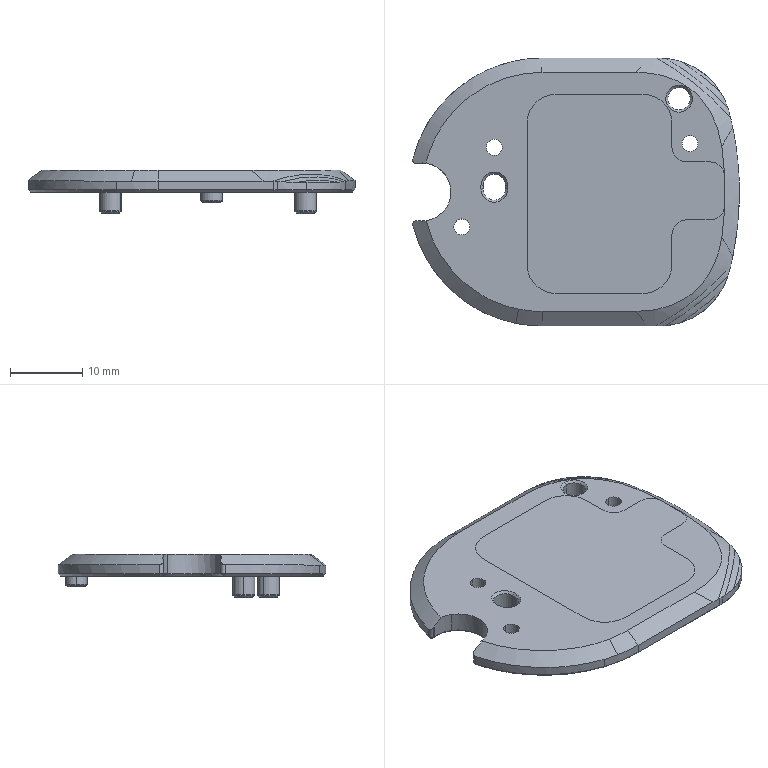NC program | NX | posted with a generic post | part box 45.101 x 36.973 x 6 mm
Lines 932 to 2608 of 3161, first 1365 of 1671 lines:
(ZLEVEL_PROFILE_COPY , TOOL : D2)
N1844 T17 M6
N1846 G54
N1848 G17 G0 G90 X-11.724 Y0.447 S9500 M3
N1850 G43 Z30. H17
N1852 Z1.5
N1854 G94 G1 Y0.253 Z1.49 F1000.
N1856 X-11.537 Y0.019 Z1.474
N1858 X-11.248 Y-0.059 Z1.458
N1860 X-10.941 Y0.074 Z1.441
N1862 X-10.824 Y0.253 Z1.429
N1864 Y1.087 Z1.386
N1866 X-10.941 Y1.266 Z1.375
N1868 X-11.247 Y1.399 Z1.357
N1870 X-11.537 Y1.322 Z1.341
N1872 X-11.724 Y1.087 Z1.326
N1874 Y0.253 Z1.282
N1876 X-11.537 Y0.019 Z1.266
N1878 X-11.248 Y-0.059 Z1.25
N1880 X-10.941 Y0.074 Z1.233
N1882 X-10.824 Y0.253 Z1.222
N1884 Y1.087 Z1.178
N1886 X-10.941 Y1.266 Z1.167
N1888 X-11.247 Y1.399 Z1.149
N1890 X-11.537 Y1.322 Z1.134
N1892 X-11.724 Y1.087 Z1.118
N1894 Y0.253 Z1.074
N1896 X-11.537 Y0.019 Z1.058
N1898 X-11.248 Y-0.059 Z1.043
N1900 X-10.941 Y0.074 Z1.025
N1902 X-10.824 Y0.253 Z1.014
N1904 Y1.087 Z0.97
N1906 X-10.941 Y1.266 Z0.959
N1908 X-11.247 Y1.399 Z0.942
N1910 X-11.537 Y1.322 Z0.926
N1912 X-11.724 Y1.087 Z0.91
N1914 Y0.253 Z0.866
N1916 X-11.537 Y0.019 Z0.851
N1918 X-11.248 Y-0.059 Z0.835
N1920 X-10.941 Y0.074 Z0.818
N1922 X-10.824 Y0.253 Z0.806
N1924 Y1.087 Z0.763
N1926 X-10.941 Y1.266 Z0.751
N1928 X-11.247 Y1.399 Z0.734
N1930 X-11.537 Y1.322 Z0.718
N1932 X-11.724 Y1.087 Z0.702
N1934 Y0.253 Z0.659
N1936 X-11.537 Y0.019 Z0.643
N1938 X-11.248 Y-0.059 Z0.627
N1940 X-10.941 Y0.074 Z0.61
N1942 X-10.824 Y0.253 Z0.599
N1944 Y1.087 Z0.555
N1946 X-10.941 Y1.266 Z0.544
N1948 X-11.247 Y1.399 Z0.526
N1950 X-11.537 Y1.322 Z0.511
N1952 X-11.724 Y1.087 Z0.495
N1954 Y0.253 Z0.451
N1956 X-11.537 Y0.019 Z0.435
N1958 X-11.248 Y-0.059 Z0.42
N1960 X-10.941 Y0.074 Z0.402
N1962 X-10.824 Y0.253 Z0.391
N1964 Y1.087 Z0.347
N1966 X-10.941 Y1.266 Z0.336
N1968 X-11.247 Y1.399 Z0.319
N1970 X-11.537 Y1.322 Z0.303
N1972 X-11.724 Y1.087 Z0.287
N1974 Y0.253 Z0.243
N1976 X-11.537 Y0.019 Z0.228
N1978 X-11.248 Y-0.059 Z0.212
N1980 X-10.941 Y0.074 Z0.194
N1982 X-10.824 Y0.253 Z0.183
N1984 Y1.087 Z0.14
N1986 X-10.941 Y1.266 Z0.128
N1988 X-11.247 Y1.399 Z0.111
N1990 X-11.537 Y1.322 Z0.095
N1992 X-11.724 Y1.087 Z0.079
N1994 Y0.253 Z0.036
N1996 X-11.537 Y0.019 Z0.02
N1998 X-11.248 Y-0.059 Z0.004
N2000 X-10.941 Y0.074 Z-0.013
N2002 X-10.824 Y0.253 Z-0.024
N2004 Y1.087 Z-0.068
N2006 X-10.941 Y1.266 Z-0.079
N2008 X-11.247 Y1.399 Z-0.097
N2010 X-11.537 Y1.322 Z-0.113
N2012 X-11.724 Y1.087 Z-0.128
N2014 Y0.67 Z-0.15
N2016 Y0.42 F1200.
N2018 G3 X-11.274 Y-0.03 R0.45
N2020 X-10.824 Y0.42 R0.45
N2022 G1 Y0.92
N2024 G3 X-11.274 Y1.37 R0.45
N2026 X-11.724 Y0.92 R0.45
N2028 G1 Y0.67
N2030 X-11.703 Y0.42 Z-0.163
N2032 X-11.692 Y0.356 Z-0.167
N2034 X-11.614 Y0.17 Z-0.178
N2036 X-11.551 Y0.097 Z-0.184
N2038 X-11.392 Y0.013 Z-0.193
N2040 X-11.274 Y-0.011 Z-0.2
N2042 X-11.111 Y0.022 Z-0.209
N2044 X-10.997 Y0.097 Z-0.217
N2046 X-10.912 Y0.202 Z-0.224
N2048 X-10.857 Y0.356 Z-0.234
N2050 X-10.83 Y0.498 Z-0.241
N2052 X-10.824 Y0.67 Z-0.25
N2054 Y0.909 Z-0.263
N2056 X-10.857 Y0.985 Z-0.267
N2058 X-10.967 Y1.219 Z-0.281
N2060 X-10.997 Y1.243 Z-0.284
N2062 X-11.13 Y1.322 Z-0.292
N2064 X-11.274 Y1.37 Z-0.3
N2066 G3 X-11.724 Y0.92 R0.45
N2068 G1 Y0.67
N2070 X-11.703 Y0.42 Z-0.313
N2072 X-11.692 Y0.356 Z-0.317
N2074 X-11.614 Y0.17 Z-0.328
N2076 X-11.551 Y0.097 Z-0.334
N2078 X-11.392 Y0.013 Z-0.343
N2080 X-11.274 Y-0.011 Z-0.35
N2082 X-11.111 Y0.022 Z-0.359
N2084 X-10.997 Y0.097 Z-0.367
N2086 X-10.912 Y0.202 Z-0.374
N2088 X-10.857 Y0.356 Z-0.384
N2090 X-10.83 Y0.498 Z-0.391
N2092 X-10.824 Y0.67 Z-0.4
N2094 Y0.909 Z-0.413
N2096 X-10.857 Y0.985 Z-0.417
N2098 X-10.967 Y1.219 Z-0.431
N2100 X-10.997 Y1.243 Z-0.434
N2102 X-11.13 Y1.322 Z-0.442
N2104 X-11.274 Y1.37 Z-0.45
N2106 G3 X-11.724 Y0.92 R0.45
N2108 G1 Y0.67
N2110 X-11.703 Y0.42 Z-0.463
N2112 X-11.692 Y0.356 Z-0.467
N2114 X-11.614 Y0.17 Z-0.478
N2116 X-11.551 Y0.097 Z-0.484
N2118 X-11.392 Y0.013 Z-0.493
N2120 X-11.274 Y-0.011 Z-0.5
N2122 X-11.111 Y0.022 Z-0.509
N2124 X-10.997 Y0.097 Z-0.517
N2126 X-10.912 Y0.202 Z-0.524
N2128 X-10.857 Y0.356 Z-0.534
N2130 X-10.83 Y0.498 Z-0.541
N2132 X-10.824 Y0.67 Z-0.55
N2134 Y0.909 Z-0.563
N2136 X-10.857 Y0.985 Z-0.567
N2138 X-10.967 Y1.219 Z-0.581
N2140 X-10.997 Y1.243 Z-0.584
N2142 X-11.13 Y1.322 Z-0.592
N2144 X-11.274 Y1.37 Z-0.6
N2146 G3 X-11.724 Y0.92 R0.45
N2148 G1 Y0.67
N2150 X-11.703 Y0.42 Z-0.613
N2152 X-11.692 Y0.356 Z-0.617
N2154 X-11.614 Y0.17 Z-0.628
N2156 X-11.551 Y0.097 Z-0.634
N2158 X-11.392 Y0.013 Z-0.643
N2160 X-11.274 Y-0.011 Z-0.65
N2162 X-11.111 Y0.022 Z-0.659
N2164 X-10.997 Y0.097 Z-0.667
N2166 X-10.912 Y0.202 Z-0.674
N2168 X-10.857 Y0.356 Z-0.684
N2170 X-10.83 Y0.498 Z-0.691
N2172 X-10.824 Y0.67 Z-0.7
N2174 Y0.909 Z-0.713
N2176 X-10.857 Y0.985 Z-0.717
N2178 X-10.967 Y1.219 Z-0.731
N2180 X-10.997 Y1.243 Z-0.734
N2182 X-11.13 Y1.322 Z-0.742
N2184 X-11.274 Y1.37 Z-0.75
N2186 G3 X-11.724 Y0.92 R0.45
N2188 G1 Y0.67
N2190 X-11.703 Y0.42 Z-0.763
N2192 X-11.692 Y0.356 Z-0.767
N2194 X-11.614 Y0.17 Z-0.778
N2196 X-11.551 Y0.097 Z-0.784
N2198 X-11.392 Y0.013 Z-0.793
N2200 X-11.274 Y-0.011 Z-0.8
N2202 X-11.111 Y0.022 Z-0.809
N2204 X-10.997 Y0.097 Z-0.817
N2206 X-10.912 Y0.202 Z-0.824
N2208 X-10.857 Y0.356 Z-0.834
N2210 X-10.83 Y0.498 Z-0.841
N2212 X-10.824 Y0.67 Z-0.85
N2214 Y0.909 Z-0.863
N2216 X-10.857 Y0.985 Z-0.867
N2218 X-10.967 Y1.219 Z-0.881
N2220 X-10.997 Y1.243 Z-0.884
N2222 X-11.13 Y1.322 Z-0.892
N2224 X-11.274 Y1.37 Z-0.9
N2226 G3 X-11.724 Y0.92 R0.45
N2228 G1 Y0.67
N2230 X-11.703 Y0.42 Z-0.913
N2232 X-11.692 Y0.356 Z-0.917
N2234 X-11.614 Y0.17 Z-0.928
N2236 X-11.551 Y0.097 Z-0.934
N2238 X-11.392 Y0.013 Z-0.943
N2240 X-11.274 Y-0.011 Z-0.95
N2242 X-11.111 Y0.022 Z-0.959
N2244 X-10.997 Y0.097 Z-0.967
N2246 X-10.912 Y0.202 Z-0.974
N2248 X-10.857 Y0.356 Z-0.984
N2250 X-10.83 Y0.498 Z-0.991
N2252 X-10.824 Y0.67 Z-1.
N2254 Y0.909 Z-1.013
N2256 X-10.857 Y0.985 Z-1.017
N2258 X-10.967 Y1.219 Z-1.031
N2260 X-10.997 Y1.243 Z-1.034
N2262 X-11.13 Y1.322 Z-1.042
N2264 X-11.274 Y1.37 Z-1.05
N2266 G3 X-11.724 Y0.92 R0.45
N2268 G1 Y0.67
N2270 X-11.703 Y0.42 Z-1.063
N2272 X-11.692 Y0.356 Z-1.067
N2274 X-11.614 Y0.17 Z-1.078
N2276 X-11.551 Y0.097 Z-1.084
N2278 X-11.392 Y0.013 Z-1.093
N2280 X-11.274 Y-0.011 Z-1.1
N2282 X-11.111 Y0.022 Z-1.109
N2284 X-10.997 Y0.097 Z-1.117
N2286 X-10.912 Y0.202 Z-1.124
N2288 X-10.857 Y0.356 Z-1.134
N2290 X-10.83 Y0.498 Z-1.141
N2292 X-10.824 Y0.67 Z-1.15
N2294 Y0.909 Z-1.163
N2296 X-10.857 Y0.985 Z-1.167
N2298 X-10.967 Y1.219 Z-1.181
N2300 X-10.997 Y1.243 Z-1.184
N2302 X-11.13 Y1.322 Z-1.192
N2304 X-11.274 Y1.37 Z-1.2
N2306 G3 X-11.724 Y0.92 R0.45
N2308 G1 Y0.67
N2310 X-11.703 Y0.42 Z-1.213
N2312 X-11.692 Y0.356 Z-1.217
N2314 X-11.614 Y0.17 Z-1.228
N2316 X-11.551 Y0.097 Z-1.234
N2318 X-11.392 Y0.013 Z-1.243
N2320 X-11.274 Y-0.011 Z-1.25
N2322 X-11.111 Y0.022 Z-1.259
N2324 X-10.997 Y0.097 Z-1.267
N2326 X-10.912 Y0.202 Z-1.274
N2328 X-10.857 Y0.356 Z-1.284
N2330 X-10.83 Y0.498 Z-1.291
N2332 X-10.824 Y0.67 Z-1.3
N2334 Y0.909 Z-1.313
N2336 X-10.857 Y0.985 Z-1.317
N2338 X-10.967 Y1.219 Z-1.331
N2340 X-10.997 Y1.243 Z-1.334
N2342 X-11.13 Y1.322 Z-1.342
N2344 X-11.274 Y1.37 Z-1.35
N2346 G3 X-11.724 Y0.92 R0.45
N2348 G1 Y0.67
N2350 X-11.703 Y0.42 Z-1.363
N2352 X-11.692 Y0.356 Z-1.367
N2354 X-11.614 Y0.17 Z-1.378
N2356 X-11.551 Y0.097 Z-1.384
N2358 X-11.392 Y0.013 Z-1.393
N2360 X-11.274 Y-0.011 Z-1.4
N2362 X-11.111 Y0.022 Z-1.409
N2364 X-10.997 Y0.097 Z-1.417
N2366 X-10.912 Y0.202 Z-1.424
N2368 X-10.857 Y0.356 Z-1.434
N2370 X-10.83 Y0.498 Z-1.441
N2372 X-10.824 Y0.67 Z-1.45
N2374 Y0.909 Z-1.463
N2376 X-10.857 Y0.985 Z-1.467
N2378 X-10.967 Y1.219 Z-1.481
N2380 X-10.997 Y1.243 Z-1.484
N2382 X-11.13 Y1.322 Z-1.492
N2384 X-11.274 Y1.37 Z-1.5
N2386 G3 X-11.724 Y0.92 R0.45
N2388 G1 Y0.67
N2390 X-11.703 Y0.42 Z-1.513
N2392 X-11.692 Y0.356 Z-1.517
N2394 X-11.614 Y0.17 Z-1.528
N2396 X-11.551 Y0.097 Z-1.534
N2398 X-11.392 Y0.013 Z-1.543
N2400 X-11.274 Y-0.011 Z-1.55
N2402 X-11.111 Y0.022 Z-1.559
N2404 X-10.997 Y0.097 Z-1.567
N2406 X-10.912 Y0.202 Z-1.574
N2408 X-10.857 Y0.356 Z-1.584
N2410 X-10.83 Y0.498 Z-1.591
N2412 X-10.824 Y0.67 Z-1.6
N2414 Y0.909 Z-1.613
N2416 X-10.857 Y0.985 Z-1.617
N2418 X-10.967 Y1.219 Z-1.631
N2420 X-10.997 Y1.243 Z-1.634
N2422 X-11.13 Y1.322 Z-1.642
N2424 X-11.274 Y1.37 Z-1.65
N2426 G3 X-11.724 Y0.92 R0.45
N2428 G1 Y0.67
N2430 X-11.703 Y0.42 Z-1.663
N2432 X-11.692 Y0.356 Z-1.667
N2434 X-11.614 Y0.17 Z-1.678
N2436 X-11.551 Y0.097 Z-1.684
N2438 X-11.392 Y0.013 Z-1.693
N2440 X-11.274 Y-0.011 Z-1.7
N2442 X-11.111 Y0.022 Z-1.709
N2444 X-10.997 Y0.097 Z-1.717
N2446 X-10.912 Y0.202 Z-1.724
N2448 X-10.857 Y0.356 Z-1.734
N2450 X-10.83 Y0.498 Z-1.741
N2452 X-10.824 Y0.67 Z-1.75
N2454 Y0.909 Z-1.763
N2456 X-10.857 Y0.985 Z-1.767
N2458 X-10.967 Y1.219 Z-1.781
N2460 X-10.997 Y1.243 Z-1.784
N2462 X-11.13 Y1.322 Z-1.792
N2464 X-11.274 Y1.37 Z-1.8
N2466 G3 X-11.724 Y0.92 R0.45
N2468 G1 Y0.67
N2470 X-11.703 Y0.42 Z-1.813
N2472 X-11.692 Y0.356 Z-1.817
N2474 X-11.614 Y0.17 Z-1.828
N2476 X-11.551 Y0.097 Z-1.834
N2478 X-11.392 Y0.013 Z-1.843
N2480 X-11.274 Y-0.011 Z-1.85
N2482 X-11.111 Y0.022 Z-1.859
N2484 X-10.997 Y0.097 Z-1.867
N2486 X-10.912 Y0.202 Z-1.874
N2488 X-10.857 Y0.356 Z-1.884
N2490 X-10.83 Y0.498 Z-1.891
N2492 X-10.824 Y0.67 Z-1.9
N2494 Y0.909 Z-1.913
N2496 X-10.857 Y0.985 Z-1.917
N2498 X-10.967 Y1.219 Z-1.931
N2500 X-10.997 Y1.243 Z-1.934
N2502 X-11.13 Y1.322 Z-1.942
N2504 X-11.274 Y1.37 Z-1.95
N2506 G3 X-11.724 Y0.92 R0.45
N2508 G1 Y0.67
N2510 X-11.703 Y0.42 Z-1.963
N2512 X-11.692 Y0.356 Z-1.967
N2514 X-11.614 Y0.17 Z-1.978
N2516 X-11.551 Y0.097 Z-1.984
N2518 X-11.392 Y0.013 Z-1.993
N2520 X-11.274 Y-0.011 Z-2.
N2522 X-11.111 Y0.022 Z-2.009
N2524 X-10.997 Y0.097 Z-2.017
N2526 X-10.912 Y0.202 Z-2.024
N2528 X-10.857 Y0.356 Z-2.034
N2530 X-10.83 Y0.498 Z-2.041
N2532 X-10.824 Y0.67 Z-2.05
N2534 Y0.909 Z-2.063
N2536 X-10.857 Y0.985 Z-2.067
N2538 X-10.967 Y1.219 Z-2.081
N2540 X-10.997 Y1.243 Z-2.084
N2542 X-11.13 Y1.322 Z-2.092
N2544 X-11.274 Y1.37 Z-2.1
N2546 G3 X-11.724 Y0.92 R0.45
N2548 G1 Y0.67
N2550 X-11.703 Y0.42 Z-2.113
N2552 X-11.692 Y0.356 Z-2.117
N2554 X-11.614 Y0.17 Z-2.128
N2556 X-11.551 Y0.097 Z-2.134
N2558 X-11.392 Y0.013 Z-2.143
N2560 X-11.274 Y-0.011 Z-2.15
N2562 X-11.111 Y0.022 Z-2.159
N2564 X-10.997 Y0.097 Z-2.167
N2566 X-10.912 Y0.202 Z-2.174
N2568 X-10.857 Y0.356 Z-2.184
N2570 X-10.83 Y0.498 Z-2.191
N2572 X-10.824 Y0.67 Z-2.2
N2574 Y0.909 Z-2.213
N2576 X-10.857 Y0.985 Z-2.217
N2578 X-10.967 Y1.219 Z-2.231
N2580 X-10.997 Y1.243 Z-2.234
N2582 X-11.13 Y1.322 Z-2.242
N2584 X-11.274 Y1.37 Z-2.25
N2586 G3 X-11.724 Y0.92 R0.45
N2588 G1 Y0.67
N2590 X-11.703 Y0.42 Z-2.263
N2592 X-11.692 Y0.356 Z-2.267
N2594 X-11.614 Y0.17 Z-2.278
N2596 X-11.551 Y0.097 Z-2.284
N2598 X-11.392 Y0.013 Z-2.293
N2600 X-11.274 Y-0.011 Z-2.3
N2602 X-11.111 Y0.022 Z-2.309
N2604 X-10.997 Y0.097 Z-2.317
N2606 X-10.912 Y0.202 Z-2.324
N2608 X-10.857 Y0.356 Z-2.334
N2610 X-10.83 Y0.498 Z-2.341
N2612 X-10.824 Y0.67 Z-2.35
N2614 Y0.909 Z-2.363
N2616 X-10.857 Y0.985 Z-2.367
N2618 X-10.967 Y1.219 Z-2.381
N2620 X-10.997 Y1.243 Z-2.384
N2622 X-11.13 Y1.322 Z-2.392
N2624 X-11.274 Y1.37 Z-2.4
N2626 G3 X-11.724 Y0.92 R0.45
N2628 G1 Y0.67
N2630 X-11.703 Y0.42 Z-2.413
N2632 X-11.692 Y0.356 Z-2.417
N2634 X-11.614 Y0.17 Z-2.428
N2636 X-11.551 Y0.097 Z-2.434
N2638 X-11.392 Y0.013 Z-2.443
N2640 X-11.274 Y-0.011 Z-2.45
N2642 X-11.111 Y0.022 Z-2.459
N2644 X-10.997 Y0.097 Z-2.467
N2646 X-10.912 Y0.202 Z-2.474
N2648 X-10.857 Y0.356 Z-2.484
N2650 X-10.83 Y0.498 Z-2.491
N2652 X-10.824 Y0.67 Z-2.5
N2654 Y0.909 Z-2.513
N2656 X-10.857 Y0.985 Z-2.517
N2658 X-10.967 Y1.219 Z-2.531
N2660 X-10.997 Y1.243 Z-2.534
N2662 X-11.13 Y1.322 Z-2.542
N2664 X-11.274 Y1.37 Z-2.55
N2666 G3 X-11.724 Y0.92 R0.45
N2668 G1 Y0.67
N2670 X-11.703 Y0.42 Z-2.563
N2672 X-11.692 Y0.356 Z-2.567
N2674 X-11.614 Y0.17 Z-2.578
N2676 X-11.551 Y0.097 Z-2.584
N2678 X-11.392 Y0.013 Z-2.593
N2680 X-11.274 Y-0.011 Z-2.6
N2682 X-11.111 Y0.022 Z-2.609
N2684 X-10.997 Y0.097 Z-2.617
N2686 X-10.912 Y0.202 Z-2.624
N2688 X-10.857 Y0.356 Z-2.634
N2690 X-10.83 Y0.498 Z-2.641
N2692 X-10.824 Y0.67 Z-2.65
N2694 Y0.909 Z-2.663
N2696 X-10.857 Y0.985 Z-2.667
N2698 X-10.967 Y1.219 Z-2.681
N2700 X-10.997 Y1.243 Z-2.684
N2702 X-11.13 Y1.322 Z-2.692
N2704 X-11.274 Y1.37 Z-2.7
N2706 G3 X-11.724 Y0.92 R0.45
N2708 G1 Y0.67
N2710 X-11.703 Y0.42 Z-2.713
N2712 X-11.692 Y0.356 Z-2.717
N2714 X-11.614 Y0.17 Z-2.728
N2716 X-11.551 Y0.097 Z-2.734
N2718 X-11.392 Y0.013 Z-2.743
N2720 X-11.274 Y-0.011 Z-2.75
N2722 X-11.111 Y0.022 Z-2.759
N2724 X-10.997 Y0.097 Z-2.767
N2726 X-10.912 Y0.202 Z-2.774
N2728 X-10.857 Y0.356 Z-2.784
N2730 X-10.83 Y0.498 Z-2.791
N2732 X-10.824 Y0.67 Z-2.8
N2734 Y0.909 Z-2.813
N2736 X-10.857 Y0.985 Z-2.817
N2738 X-10.967 Y1.219 Z-2.831
N2740 X-10.997 Y1.243 Z-2.834
N2742 X-11.13 Y1.322 Z-2.842
N2744 X-11.274 Y1.37 Z-2.85
N2746 G3 X-11.724 Y0.92 R0.45
N2748 G1 Y0.67
N2750 X-11.703 Y0.42 Z-2.863
N2752 X-11.692 Y0.356 Z-2.867
N2754 X-11.614 Y0.17 Z-2.878
N2756 X-11.551 Y0.097 Z-2.884
N2758 X-11.392 Y0.013 Z-2.893
N2760 X-11.274 Y-0.011 Z-2.9
N2762 X-11.111 Y0.022 Z-2.909
N2764 X-10.997 Y0.097 Z-2.917
N2766 X-10.912 Y0.202 Z-2.924
N2768 X-10.857 Y0.356 Z-2.934
N2770 X-10.83 Y0.498 Z-2.941
N2772 X-10.824 Y0.67 Z-2.95
N2774 Y0.909 Z-2.963
N2776 X-10.857 Y0.985 Z-2.967
N2778 X-10.967 Y1.219 Z-2.981
N2780 X-10.997 Y1.243 Z-2.984
N2782 X-11.13 Y1.322 Z-2.992
N2784 X-11.274 Y1.37 Z-3.
N2786 G3 X-11.724 Y0.92 R0.45
N2788 G1 Y0.42
N2790 G3 X-11.274 Y-0.03 R0.45
N2792 X-10.824 Y0.42 R0.45
N2794 G1 Y0.92
N2796 G3 X-11.274 Y1.37 R0.45
N2798 G1 Z-1.5
N2800 G0 Z30.
N2802 X13.893 Y12.55
N2804 Z1.5
N2806 G1 X14.081 Y12.412 Z1.488 F1000.
N2808 X14.415 Y12.429 Z1.47
N2810 X14.633 Y12.615 Z1.455
N2812 X14.705 Y12.892 Z1.44
N2814 X14.575 Y13.2 Z1.423
N2816 X14.415 Y13.311 Z1.412
N2818 X14.226 Y13.32 Z1.402
N2820 X14.059 Z1.394
N2822 X13.877 Y13.2 Z1.382
N2824 X13.746 Y12.892 Z1.365
N2826 X13.832 Y12.595 Z1.349
N2828 X14.081 Y12.412 Z1.332
N2830 X14.415 Y12.429 Z1.315
N2832 X14.633 Y12.615 Z1.3
N2834 X14.705 Y12.892 Z1.285
N2836 X14.575 Y13.2 Z1.267
N2838 X14.415 Y13.311 Z1.257
N2840 X14.226 Y13.32 Z1.247
N2842 X14.059 Z1.238
N2844 X13.877 Y13.2 Z1.227
N2846 X13.746 Y12.892 Z1.209
N2848 X13.832 Y12.595 Z1.193
N2850 X14.081 Y12.412 Z1.177
N2852 X14.415 Y12.429 Z1.16
N2854 X14.633 Y12.615 Z1.145
N2856 X14.705 Y12.892 Z1.13
N2858 X14.575 Y13.2 Z1.112
N2860 X14.415 Y13.311 Z1.102
N2862 X14.226 Y13.32 Z1.092
N2864 X14.059 Z1.083
N2866 X13.877 Y13.2 Z1.072
N2868 X13.746 Y12.892 Z1.054
N2870 X13.832 Y12.595 Z1.038
N2872 X14.081 Y12.412 Z1.022
N2874 X14.415 Y12.429 Z1.004
N2876 X14.633 Y12.615 Z0.989
N2878 X14.705 Y12.892 Z0.974
N2880 X14.575 Y13.2 Z0.957
N2882 X14.415 Y13.311 Z0.947
N2884 X14.226 Y13.32 Z0.937
N2886 X14.059 Z0.928
N2888 X13.877 Y13.2 Z0.916
N2890 X13.746 Y12.892 Z0.899
N2892 X13.832 Y12.595 Z0.883
N2894 X14.081 Y12.412 Z0.867
N2896 X14.415 Y12.429 Z0.849
N2898 X14.633 Y12.615 Z0.834
N2900 X14.705 Y12.892 Z0.819
N2902 X14.575 Y13.2 Z0.801
N2904 X14.415 Y13.311 Z0.791
N2906 X14.226 Y13.32 Z0.781
N2908 X14.059 Z0.773
N2910 X13.877 Y13.2 Z0.761
N2912 X13.746 Y12.892 Z0.744
N2914 X13.832 Y12.595 Z0.727
N2916 X14.081 Y12.412 Z0.711
N2918 X14.415 Y12.429 Z0.694
N2920 X14.633 Y12.615 Z0.679
N2922 X14.705 Y12.892 Z0.664
N2924 X14.575 Y13.2 Z0.646
N2926 X14.415 Y13.311 Z0.636
N2928 X14.226 Y13.32 Z0.626
N2930 X14.059 Z0.617
N2932 X13.877 Y13.2 Z0.606
N2934 X13.746 Y12.892 Z0.588
N2936 X13.832 Y12.595 Z0.572
N2938 X14.081 Y12.412 Z0.556
N2940 X14.415 Y12.429 Z0.539
N2942 X14.633 Y12.615 Z0.524
N2944 X14.705 Y12.892 Z0.508
N2946 X14.575 Y13.2 Z0.491
N2948 X14.415 Y13.311 Z0.481
N2950 X14.226 Y13.32 Z0.471
N2952 X14.059 Z0.462
N2954 X13.877 Y13.2 Z0.451
N2956 X13.746 Y12.892 Z0.433
N2958 X13.832 Y12.595 Z0.417
N2960 X14.081 Y12.412 Z0.401
N2962 X14.415 Y12.429 Z0.383
N2964 X14.633 Y12.615 Z0.368
N2966 X14.705 Y12.892 Z0.353
N2968 X14.575 Y13.2 Z0.336
N2970 X14.415 Y13.311 Z0.325
N2972 X14.226 Y13.32 Z0.316
N2974 X14.059 Z0.307
N2976 X13.877 Y13.2 Z0.295
N2978 X13.746 Y12.892 Z0.278
N2980 X13.832 Y12.595 Z0.262
N2982 X14.081 Y12.412 Z0.246
N2984 X14.415 Y12.429 Z0.228
N2986 X14.633 Y12.615 Z0.213
N2988 X14.705 Y12.892 Z0.198
N2990 X14.575 Y13.2 Z0.18
N2992 X14.415 Y13.311 Z0.17
N2994 X14.226 Y13.32 Z0.16
N2996 X14.059 Z0.152
N2998 X13.877 Y13.2 Z0.14
N3000 X13.746 Y12.892 Z0.123
N3002 X13.832 Y12.595 Z0.106
N3004 X14.081 Y12.412 Z0.09
N3006 X14.415 Y12.429 Z0.073
N3008 X14.633 Y12.615 Z0.058
N3010 X14.705 Y12.892 Z0.043
N3012 X14.575 Y13.2 Z0.025
N3014 X14.415 Y13.311 Z0.015
N3016 X14.226 Y13.32 Z0.005
N3018 X14.059 Z-0.004
N3020 X13.877 Y13.2 Z-0.015
N3022 X13.746 Y12.892 Z-0.033
N3024 X13.832 Y12.595 Z-0.049
N3026 X14.081 Y12.412 Z-0.065
N3028 X14.415 Y12.429 Z-0.083
N3030 X14.633 Y12.615 Z-0.098
N3032 X14.705 Y12.892 Z-0.113
N3034 X14.575 Y13.2 Z-0.13
N3036 X14.415 Y13.311 Z-0.14
N3038 X14.226 Y13.32 Z-0.15
N3040 G3 X13.776 Y12.87 R0.45 F1200.
N3042 X14.226 Y13.32 R-0.45
N3044 G1 X14.064 Y13.269 Z-0.163
N3046 X13.961 Y13.202 Z-0.172
N3048 X13.853 Y13.071 Z-0.184
N3050 X13.814 Y12.964 Z-0.193
N3052 X13.811 Y12.794 Z-0.206
N3054 X13.841 Y12.685 Z-0.214
N3056 X13.938 Y12.555 Z-0.227
N3058 X14.041 Y12.486 Z-0.236
N3060 X14.197 Y12.445 Z-0.248
N3062 X14.32 Y12.458 Z-0.257
N3064 X14.466 Y12.523 Z-0.269
N3066 X14.557 Y12.606 Z-0.279
N3068 X14.629 Y12.734 Z-0.289
N3070 X14.676 Y12.87 Z-0.3
N3072 G3 X14.226 Y13.32 R0.45
N3074 G1 X14.064 Y13.269 Z-0.313
N3076 X13.961 Y13.202 Z-0.322
N3078 X13.853 Y13.071 Z-0.334
N3080 X13.814 Y12.964 Z-0.343
N3082 X13.811 Y12.794 Z-0.356
N3084 X13.841 Y12.685 Z-0.364
N3086 X13.938 Y12.555 Z-0.377
N3088 X14.041 Y12.486 Z-0.386
N3090 X14.197 Y12.445 Z-0.398
N3092 X14.32 Y12.458 Z-0.407
N3094 X14.466 Y12.523 Z-0.419
N3096 X14.557 Y12.606 Z-0.429
N3098 X14.629 Y12.734 Z-0.439
N3100 X14.676 Y12.87 Z-0.45
N3102 G3 X14.226 Y13.32 R0.45
N3104 G1 X14.064 Y13.269 Z-0.463
N3106 X13.961 Y13.202 Z-0.472
N3108 X13.853 Y13.071 Z-0.484
N3110 X13.814 Y12.964 Z-0.493
N3112 X13.811 Y12.794 Z-0.506
N3114 X13.841 Y12.685 Z-0.514
N3116 X13.938 Y12.555 Z-0.527
N3118 X14.041 Y12.486 Z-0.536
N3120 X14.197 Y12.445 Z-0.548
N3122 X14.32 Y12.458 Z-0.557
N3124 X14.466 Y12.523 Z-0.569
N3126 X14.557 Y12.606 Z-0.579
N3128 X14.629 Y12.734 Z-0.589
N3130 X14.676 Y12.87 Z-0.6
N3132 G3 X14.226 Y13.32 R0.45
N3134 G1 X14.064 Y13.269 Z-0.613
N3136 X13.961 Y13.202 Z-0.622
N3138 X13.853 Y13.071 Z-0.634
N3140 X13.814 Y12.964 Z-0.643
N3142 X13.811 Y12.794 Z-0.656
N3144 X13.841 Y12.685 Z-0.664
N3146 X13.938 Y12.555 Z-0.677
N3148 X14.041 Y12.486 Z-0.686
N3150 X14.197 Y12.445 Z-0.698
N3152 X14.32 Y12.458 Z-0.707
N3154 X14.466 Y12.523 Z-0.719
N3156 X14.557 Y12.606 Z-0.729
N3158 X14.629 Y12.734 Z-0.739
N3160 X14.676 Y12.87 Z-0.75
N3162 G3 X14.226 Y13.32 R0.45
N3164 G1 X14.064 Y13.269 Z-0.763
N3166 X13.961 Y13.202 Z-0.772
N3168 X13.853 Y13.071 Z-0.784
N3170 X13.814 Y12.964 Z-0.793
N3172 X13.811 Y12.794 Z-0.806
N3174 X13.841 Y12.685 Z-0.814
N3176 X13.938 Y12.555 Z-0.827
N3178 X14.041 Y12.486 Z-0.836
N3180 X14.197 Y12.445 Z-0.848
N3182 X14.32 Y12.458 Z-0.857
N3184 X14.466 Y12.523 Z-0.869
N3186 X14.557 Y12.606 Z-0.879
N3188 X14.629 Y12.734 Z-0.889
N3190 X14.676 Y12.87 Z-0.9
N3192 G3 X14.226 Y13.32 R0.45
N3194 G1 X14.064 Y13.269 Z-0.913
N3196 X13.961 Y13.202 Z-0.922
N3198 X13.853 Y13.071 Z-0.934
N3200 X13.814 Y12.964 Z-0.943
N3202 X13.811 Y12.794 Z-0.956
N3204 X13.841 Y12.685 Z-0.964
N3206 X13.938 Y12.555 Z-0.977
N3208 X14.041 Y12.486 Z-0.986
N3210 X14.197 Y12.445 Z-0.998
N3212 X14.32 Y12.458 Z-1.007
N3214 X14.466 Y12.523 Z-1.019
N3216 X14.557 Y12.606 Z-1.029
N3218 X14.629 Y12.734 Z-1.039
N3220 X14.676 Y12.87 Z-1.05
N3222 G3 X14.226 Y13.32 R0.45
N3224 G1 X14.064 Y13.269 Z-1.063
N3226 X13.961 Y13.202 Z-1.072
N3228 X13.853 Y13.071 Z-1.084
N3230 X13.814 Y12.964 Z-1.093
N3232 X13.811 Y12.794 Z-1.106
N3234 X13.841 Y12.685 Z-1.114
N3236 X13.938 Y12.555 Z-1.127
N3238 X14.041 Y12.486 Z-1.136
N3240 X14.197 Y12.445 Z-1.148
N3242 X14.32 Y12.458 Z-1.157
N3244 X14.466 Y12.523 Z-1.169
N3246 X14.557 Y12.606 Z-1.179
N3248 X14.629 Y12.734 Z-1.189
N3250 X14.676 Y12.87 Z-1.2
N3252 G3 X14.226 Y13.32 R0.45
N3254 G1 X14.064 Y13.269 Z-1.213
N3256 X13.961 Y13.202 Z-1.222
N3258 X13.853 Y13.071 Z-1.234
N3260 X13.814 Y12.964 Z-1.243
N3262 X13.811 Y12.794 Z-1.256
N3264 X13.841 Y12.685 Z-1.264
N3266 X13.938 Y12.555 Z-1.277
N3268 X14.041 Y12.486 Z-1.286
N3270 X14.197 Y12.445 Z-1.298
N3272 X14.32 Y12.458 Z-1.307
N3274 X14.466 Y12.523 Z-1.319
N3276 X14.557 Y12.606 Z-1.329
N3278 X14.629 Y12.734 Z-1.339
N3280 X14.676 Y12.87 Z-1.35
N3282 G3 X14.226 Y13.32 R0.45
N3284 G1 X14.064 Y13.269 Z-1.363
N3286 X13.961 Y13.202 Z-1.372
N3288 X13.853 Y13.071 Z-1.384
N3290 X13.814 Y12.964 Z-1.393
N3292 X13.811 Y12.794 Z-1.406
N3294 X13.841 Y12.685 Z-1.414
N3296 X13.938 Y12.555 Z-1.427
N3298 X14.041 Y12.486 Z-1.436
N3300 X14.197 Y12.445 Z-1.448
N3302 X14.32 Y12.458 Z-1.457
N3304 X14.466 Y12.523 Z-1.469
N3306 X14.557 Y12.606 Z-1.479
N3308 X14.629 Y12.734 Z-1.489
N3310 X14.676 Y12.87 Z-1.5
N3312 G3 X14.226 Y13.32 R0.45
N3314 G1 X14.064 Y13.269 Z-1.513
N3316 X13.961 Y13.202 Z-1.522
N3318 X13.853 Y13.071 Z-1.534
N3320 X13.814 Y12.964 Z-1.543
N3322 X13.811 Y12.794 Z-1.556
N3324 X13.841 Y12.685 Z-1.564
N3326 X13.938 Y12.555 Z-1.577
N3328 X14.041 Y12.486 Z-1.586
N3330 X14.197 Y12.445 Z-1.598
N3332 X14.32 Y12.458 Z-1.607
N3334 X14.466 Y12.523 Z-1.619
N3336 X14.557 Y12.606 Z-1.629
N3338 X14.629 Y12.734 Z-1.639
N3340 X14.676 Y12.87 Z-1.65
N3342 G3 X14.226 Y13.32 R0.45
N3344 G1 X14.064 Y13.269 Z-1.663
N3346 X13.961 Y13.202 Z-1.672
N3348 X13.853 Y13.071 Z-1.684
N3350 X13.814 Y12.964 Z-1.693
N3352 X13.811 Y12.794 Z-1.706
N3354 X13.841 Y12.685 Z-1.714
N3356 X13.938 Y12.555 Z-1.727
N3358 X14.041 Y12.486 Z-1.736
N3360 X14.197 Y12.445 Z-1.748
N3362 X14.32 Y12.458 Z-1.757
N3364 X14.466 Y12.523 Z-1.769
N3366 X14.557 Y12.606 Z-1.779
N3368 X14.629 Y12.734 Z-1.789
N3370 X14.676 Y12.87 Z-1.8
N3372 G3 X14.226 Y13.32 R0.45
N3374 G1 X14.064 Y13.269 Z-1.813
N3376 X13.961 Y13.202 Z-1.822
N3378 X13.853 Y13.071 Z-1.834
N3380 X13.814 Y12.964 Z-1.843
N3382 X13.811 Y12.794 Z-1.856
N3384 X13.841 Y12.685 Z-1.864
N3386 X13.938 Y12.555 Z-1.877
N3388 X14.041 Y12.486 Z-1.886
N3390 X14.197 Y12.445 Z-1.898
N3392 X14.32 Y12.458 Z-1.907
N3394 X14.466 Y12.523 Z-1.919
N3396 X14.557 Y12.606 Z-1.929
N3398 X14.629 Y12.734 Z-1.939
N3400 X14.676 Y12.87 Z-1.95
N3402 G3 X14.226 Y13.32 R0.45
N3404 G1 X14.064 Y13.269 Z-1.963
N3406 X13.961 Y13.202 Z-1.972
N3408 X13.853 Y13.071 Z-1.984
N3410 X13.814 Y12.964 Z-1.993
N3412 X13.811 Y12.794 Z-2.006
N3414 X13.841 Y12.685 Z-2.014
N3416 X13.938 Y12.555 Z-2.027
N3418 X14.041 Y12.486 Z-2.036
N3420 X14.197 Y12.445 Z-2.048
N3422 X14.32 Y12.458 Z-2.057
N3424 X14.466 Y12.523 Z-2.069
N3426 X14.557 Y12.606 Z-2.079
N3428 X14.629 Y12.734 Z-2.089
N3430 X14.676 Y12.87 Z-2.1
N3432 G3 X14.226 Y13.32 R0.45
N3434 G1 X14.064 Y13.269 Z-2.113
N3436 X13.961 Y13.202 Z-2.122
N3438 X13.853 Y13.071 Z-2.134
N3440 X13.814 Y12.964 Z-2.143
N3442 X13.811 Y12.794 Z-2.156
N3444 X13.841 Y12.685 Z-2.164
N3446 X13.938 Y12.555 Z-2.177
N3448 X14.041 Y12.486 Z-2.186
N3450 X14.197 Y12.445 Z-2.198
N3452 X14.32 Y12.458 Z-2.207
N3454 X14.466 Y12.523 Z-2.219
N3456 X14.557 Y12.606 Z-2.229
N3458 X14.629 Y12.734 Z-2.239
N3460 X14.676 Y12.87 Z-2.25
N3462 G3 X14.226 Y13.32 R0.45
N3464 G1 X14.064 Y13.269 Z-2.263
N3466 X13.961 Y13.202 Z-2.272
N3468 X13.853 Y13.071 Z-2.284
N3470 X13.814 Y12.964 Z-2.293
N3472 X13.811 Y12.794 Z-2.306
N3474 X13.841 Y12.685 Z-2.314
N3476 X13.938 Y12.555 Z-2.327
N3478 X14.041 Y12.486 Z-2.336
N3480 X14.197 Y12.445 Z-2.348
N3482 X14.32 Y12.458 Z-2.357
N3484 X14.466 Y12.523 Z-2.369
N3486 X14.557 Y12.606 Z-2.379
N3488 X14.629 Y12.734 Z-2.389
N3490 X14.676 Y12.87 Z-2.4
N3492 G3 X14.226 Y13.32 R0.45
N3494 G1 X14.064 Y13.269 Z-2.413
N3496 X13.961 Y13.202 Z-2.422
N3498 X13.853 Y13.071 Z-2.434
N3500 X13.814 Y12.964 Z-2.443
N3502 X13.811 Y12.794 Z-2.456
N3504 X13.841 Y12.685 Z-2.464
N3506 X13.938 Y12.555 Z-2.477
N3508 X14.041 Y12.486 Z-2.486
N3510 X14.197 Y12.445 Z-2.498
N3512 X14.32 Y12.458 Z-2.507
N3514 X14.466 Y12.523 Z-2.519
N3516 X14.557 Y12.606 Z-2.529
N3518 X14.629 Y12.734 Z-2.539
N3520 X14.676 Y12.87 Z-2.55
N3522 G3 X14.226 Y13.32 R0.45
N3524 G1 X14.064 Y13.269 Z-2.563
N3526 X13.961 Y13.202 Z-2.572
N3528 X13.853 Y13.071 Z-2.584
N3530 X13.814 Y12.964 Z-2.593
N3532 X13.811 Y12.794 Z-2.606
N3534 X13.841 Y12.685 Z-2.614
N3536 X13.938 Y12.555 Z-2.627
N3538 X14.041 Y12.486 Z-2.636
N3540 X14.197 Y12.445 Z-2.648
N3542 X14.32 Y12.458 Z-2.657
N3544 X14.466 Y12.523 Z-2.669
N3546 X14.557 Y12.606 Z-2.679
N3548 X14.629 Y12.734 Z-2.689
N3550 X14.676 Y12.87 Z-2.7
N3552 G3 X14.226 Y13.32 R0.45
N3554 G1 X14.064 Y13.269 Z-2.713
N3556 X13.961 Y13.202 Z-2.722
N3558 X13.853 Y13.071 Z-2.734
N3560 X13.814 Y12.964 Z-2.743
N3562 X13.811 Y12.794 Z-2.756
N3564 X13.841 Y12.685 Z-2.764
N3566 X13.938 Y12.555 Z-2.777
N3568 X14.041 Y12.486 Z-2.786
N3570 X14.197 Y12.445 Z-2.798
N3572 X14.32 Y12.458 Z-2.807
N3574 X14.466 Y12.523 Z-2.819
N3576 X14.557 Y12.606 Z-2.829
N3578 X14.629 Y12.734 Z-2.839
N3580 X14.676 Y12.87 Z-2.85
N3582 G3 X14.226 Y13.32 R0.45
N3584 G1 X14.064 Y13.269 Z-2.863
N3586 X13.961 Y13.202 Z-2.872
N3588 X13.853 Y13.071 Z-2.884
N3590 X13.814 Y12.964 Z-2.893
N3592 X13.811 Y12.794 Z-2.906
N3594 X13.841 Y12.685 Z-2.914
N3596 X13.938 Y12.555 Z-2.927
N3598 X14.041 Y12.486 Z-2.936
N3600 X14.197 Y12.445 Z-2.948
N3602 X14.32 Y12.458 Z-2.957
N3604 X14.466 Y12.523 Z-2.969
N3606 X14.557 Y12.606 Z-2.979
N3608 X14.629 Y12.734 Z-2.989
N3610 X14.676 Y12.87 Z-3.
N3612 G3 X14.226 Y13.32 R0.45
N3614 X14.676 Y12.87 R-0.45
N3616 G1 Z-1.5
N3618 G0 Z30.
N3620 M5
(HOLE_MILLING , TOOL : D1.5)
N3622 T16 M6
N3624 G54
N3626 G17 G0 G90 X-15.774 Y-4.83 S9500 M3
N3628 G43 Z30. H16
N3630 Z0.5
N3632 G94 G3 X-15.649 Y-4.955 R0.125 F1000.
N3634 X-15.524 Y-4.83 R0.125
N3636 X-15.524 Y-4.83 Z0.35 I-0.25 J0.
N3638 X-15.524 Y-4.83 Z0.2 I-0.25 J0.
N3640 X-15.524 Y-4.83 Z0.05 I-0.25 J0.
N3642 X-15.524 Y-4.83 Z-0.1 I-0.25 J0.
N3644 X-15.524 Y-4.83 Z-0.25 I-0.25 J0.
N3646 X-15.524 Y-4.83 Z-0.4 I-0.25 J0.
N3648 X-15.524 Y-4.83 Z-0.55 I-0.25 J0.
N3650 X-15.524 Y-4.83 Z-0.7 I-0.25 J0.
N3652 X-15.524 Y-4.83 Z-0.85 I-0.25 J0.
N3654 X-15.524 Y-4.83 Z-1. I-0.25 J0.
N3656 X-15.524 Y-4.83 Z-1.15 I-0.25 J0.
N3658 X-15.524 Y-4.83 Z-1.3 I-0.25 J0.
N3660 X-15.524 Y-4.83 Z-1.45 I-0.25 J0.
N3662 X-15.524 Y-4.83 Z-1.6 I-0.25 J0.
N3664 X-15.524 Y-4.83 Z-1.75 I-0.25 J0.
N3666 X-15.524 Y-4.83 Z-1.9 I-0.25 J0.
N3668 X-15.524 Y-4.83 Z-2.05 I-0.25 J0.
N3670 X-15.524 Y-4.83 Z-2.2 I-0.25 J0.
N3672 X-15.524 Y-4.83 Z-2.35 I-0.25 J0.
N3674 X-15.524 Y-4.83 Z-2.5 I-0.25 J0.
N3676 X-15.524 Y-4.83 Z-2.65 I-0.25 J0.
N3678 X-15.524 Y-4.83 Z-2.8 I-0.25 J0.
N3680 X-15.524 Y-4.83 Z-2.95 I-0.25 J0.
N3682 X-15.899 Y-4.613 Z-3. R0.25
N3684 X-15.991 Y-4.955 R0.25
N3686 X-15.899 Y-4.613 R-0.25
N3688 X-15.945 Y-4.784 R0.125
N3690 X-15.774 Y-4.83 R0.125
N3692 G0 Z30.
N3694 X-11.274 Y6.17
N3696 Z0.5
N3698 G3 X-11.149 Y6.045 R0.125
N3700 X-11.024 Y6.17 R0.125
N3702 X-11.024 Y6.17 Z0.35 I-0.25 J0.
N3704 X-11.024 Y6.17 Z0.2 I-0.25 J0.
N3706 X-11.024 Y6.17 Z0.05 I-0.25 J0.
N3708 X-11.024 Y6.17 Z-0.1 I-0.25 J0.
N3710 X-11.024 Y6.17 Z-0.25 I-0.25 J0.
N3712 X-11.024 Y6.17 Z-0.4 I-0.25 J0.
N3714 X-11.024 Y6.17 Z-0.55 I-0.25 J0.
N3716 X-11.024 Y6.17 Z-0.7 I-0.25 J0.
N3718 X-11.024 Y6.17 Z-0.85 I-0.25 J0.
N3720 X-11.024 Y6.17 Z-1. I-0.25 J0.
N3722 X-11.024 Y6.17 Z-1.15 I-0.25 J0.
N3724 X-11.024 Y6.17 Z-1.3 I-0.25 J0.
N3726 X-11.024 Y6.17 Z-1.45 I-0.25 J0.
N3728 X-11.024 Y6.17 Z-1.6 I-0.25 J0.
N3730 X-11.024 Y6.17 Z-1.75 I-0.25 J0.
N3732 X-11.024 Y6.17 Z-1.9 I-0.25 J0.
N3734 X-11.024 Y6.17 Z-2.05 I-0.25 J0.
N3736 X-11.024 Y6.17 Z-2.2 I-0.25 J0.
N3738 X-11.024 Y6.17 Z-2.35 I-0.25 J0.
N3740 X-11.024 Y6.17 Z-2.5 I-0.25 J0.
N3742 X-11.024 Y6.17 Z-2.65 I-0.25 J0.
N3744 X-11.024 Y6.17 Z-2.8 I-0.25 J0.
N3746 X-11.024 Y6.17 Z-2.95 I-0.25 J0.
N3748 X-11.399 Y6.387 Z-3. R0.25
N3750 X-11.491 Y6.045 R0.25
N3752 X-11.399 Y6.387 R-0.25
N3754 X-11.445 Y6.216 R0.125
N3756 X-11.274 Y6.17 R0.125
N3758 G0 Z30.
N3760 X15.726 Y6.67
N3762 Z0.5
N3764 G3 X15.851 Y6.545 R0.125
N3766 X15.976 Y6.67 R0.125
N3768 X15.976 Y6.67 Z0.35 I-0.25 J0.
N3770 X15.976 Y6.67 Z0.2 I-0.25 J0.
N3772 X15.976 Y6.67 Z0.05 I-0.25 J0.
N3774 X15.976 Y6.67 Z-0.1 I-0.25 J0.
N3776 X15.976 Y6.67 Z-0.25 I-0.25 J0.
N3778 X15.976 Y6.67 Z-0.4 I-0.25 J0.
N3780 X15.976 Y6.67 Z-0.55 I-0.25 J0.
N3782 X15.976 Y6.67 Z-0.7 I-0.25 J0.
N3784 X15.976 Y6.67 Z-0.85 I-0.25 J0.
N3786 X15.976 Y6.67 Z-1. I-0.25 J0.
N3788 X15.976 Y6.67 Z-1.15 I-0.25 J0.
N3790 X15.976 Y6.67 Z-1.3 I-0.25 J0.
N3792 X15.976 Y6.67 Z-1.45 I-0.25 J0.
N3794 X15.976 Y6.67 Z-1.6 I-0.25 J0.
N3796 X15.976 Y6.67 Z-1.75 I-0.25 J0.
N3798 X15.976 Y6.67 Z-1.9 I-0.25 J0.
N3800 X15.976 Y6.67 Z-2.05 I-0.25 J0.
N3802 X15.976 Y6.67 Z-2.2 I-0.25 J0.
N3804 X15.976 Y6.67 Z-2.35 I-0.25 J0.
N3806 X15.976 Y6.67 Z-2.5 I-0.25 J0.
N3808 X15.976 Y6.67 Z-2.65 I-0.25 J0.
N3810 X15.976 Y6.67 Z-2.8 I-0.25 J0.
N3812 X15.976 Y6.67 Z-2.95 I-0.25 J0.
N3814 X15.601 Y6.887 Z-3. R0.25
N3816 X15.509 Y6.545 R0.25
N3818 X15.601 Y6.887 R-0.25
N3820 X15.555 Y6.716 R0.125
N3822 X15.726 Y6.67 R0.125
N3824 G0 Z30.
N3826 M5
(ZLEVEL_PROFILE_1 , TOOL : D3R0.5)
N3828 T18 M6
N3830 G54
N3832 G17 G0 G90 X-22.734 Y3.123 S9500 M3
N3834 G43 Z30. H18
N3836 Z0.95
N3838 G94 G1 Z-0.05 F1000.
N3840 X-22.297 Y3.267
N3842 G3 X-22.098 Y3.492 R0.3
N3844 G2 X-13.512 Y15.397 R17.934 F3000.
N3846 X-4.711 Y17.747 R17.834
N3848 G1 X8.247 Y17.748
N3850 X8.736 Y17.74
N3852 G2 X15.374 Y15.981 R13.817
N3854 X20.459 Y9.869 R11.923
N3856 X21.452 Y5.792 R18.282
N3858 G1 X21.524 Y5.214
N3860 G2 X21.21 Y-7.265 R42.532
N3862 X17.975 Y-13.872 R13.527
N3864 X11.747 Y-17.354 R12.004
N3866 X8.247 Y-17.718 R16.896
N3868 G1 X-4.711 Y-17.719
N3870 G2 X-21.884 Y-4.329 R17.746
N3872 G1 X-22.069 Y-3.594
N3874 X-22.087 Y-3.506
N3876 X-22.125 Y-3.507 Z-0.076
N3878 X-22.155 Y-3.508 Z-0.101
N3880 X-22.137 Y-3.595
N3882 X-21.964 Y-4.294
N3884 G3 X-8.622 Y-17.348 R17.801
N3886 G1 X-8.188 Y-17.44
N3888 G3 X-4.69 Y-17.787 R17.801
N3890 G1 X8.349 Y-17.785
N3892 G3 X12.093 Y-17.348 R16.264
N3894 G1 X12.159 Y-17.333
N3896 G3 X19.004 Y-12.741 R11.676
N3898 X21.357 Y-6.872 R14.417
N3900 X21.39 Y6.678 R43.102
N3902 X20.344 Y10.353 R15.737
N3904 X14.359 Y16.6 R11.737
N3906 X8.529 Y17.816 R14.58
N3908 G1 X-4.694 Y17.814
N3910 G3 X-21.974 Y4.28 R17.801
N3912 G1 X-22.166 Y3.494
N3914 X-22.201 Y3.496 Z-0.126
N3916 X-22.234 Y3.497 Z-0.151
N3918 X-22.041 Y4.288
N3920 G2 X-4.666 Y17.881 R17.868
N3922 G1 X8.562 Y17.883
N3924 G2 X13.632 Y16.982 R14.708
N3926 X20.169 Y10.949 R11.6
N3928 X21.466 Y6.621 R16.101
N3930 X21.41 Y-6.961 R43.169
N3932 X18.997 Y-12.893 R14.397
N3934 X11.914 Y-17.469 R11.72
N3936 G1 X11.56 Y-17.543
N3938 G2 X8.328 Y-17.852 R16.411
N3940 G1 X-4.69 Y-17.854
N3942 G2 X-22.031 Y-4.301 R17.868
N3944 G1 X-22.206 Y-3.595
N3946 X-22.223 Y-3.51
N3948 X-22.261 Y-3.511 Z-0.176
N3950 X-22.292 Y-3.512 Z-0.201
N3952 X-22.274 Y-3.595
N3954 X-22.098 Y-4.308
N3956 G3 X-4.69 Y-17.921 R17.935
N3958 G1 X8.385 Y-17.919
N3960 G3 X11.914 Y-17.548 R16.515
N3962 G1 X12.159 Y-17.494
N3964 G3 X19.004 Y-13.026 R11.707
N3966 X21.462 Y-7.059 R14.357
N3968 X21.52 Y6.713 R43.236
N3970 X20.198 Y11.067 R16.009
N3972 X13.522 Y17.109 R11.617
N3974 X8.588 Y17.95 R14.893
N3976 G1 X-4.688 Y17.948
N3978 G3 X-22.108 Y4.295 R17.935
N3980 G1 X-22.303 Y3.5
N3982 X-22.337 Z-0.226
N3984 X-22.371 Z-0.251
N3986 X-22.176 Y4.302
N3988 G2 X-4.688 Y18.015 R18.002
N3990 G1 X8.436 Y18.017
N3992 G2 X13.282 Y17.278 R15.225
N3994 X20.298 Y11.04 R11.676
N3996 X21.573 Y6.805 R16.089
N3998 X21.515 Y-7.151 R43.303
N4000 X19.025 Y-13.138 R14.339
N4002 X12.159 Y-17.574 R11.725
N4004 G1 X11.914 Y-17.626
N4006 G2 X8.442 Y-17.986 R16.615
N4008 G1 X-4.69 Y-17.988
N4010 G2 X-22.166 Y-4.314 R18.002
N4012 G1 X-22.343 Y-3.595
N4014 X-22.359 Y-3.512
N4016 X-22.397 Z-0.277
N4018 X-22.428 Y-3.511 Z-0.302
N4020 X-22.411 Y-3.595
N4022 X-22.234 Y-4.318
N4024 G3 X-4.69 Y-18.055 R18.069
N4026 G1 X8.5 Y-18.053
N4028 G3 X11.914 Y-17.704 R16.644
N4030 G1 X12.159 Y-17.654
N4032 G3 X19.129 Y-13.138 R11.732
N4034 X21.569 Y-7.231 R14.376
N4036 X21.626 Y6.897 R43.37
N4038 X20.308 Y11.2 R15.98
N4040 X13.307 Y17.355 R11.667
N4042 X8.493 Y18.084 R15.288
N4044 G1 X-4.688 Y18.082
N4046 G3 X-22.243 Y4.307 R18.069
N4048 G1 X-22.439 Y3.5
N4050 X-22.473 Z-0.327
N4052 X-22.507 Z-0.352
N4054 X-22.311 Y4.311
N4056 G2 X-4.688 Y18.149 R18.136
N4058 G1 X8.551 Y18.151
N4060 G2 X13.282 Y17.448 R15.346
N4062 X20.371 Y11.247 R11.692
N4064 X21.679 Y6.99 R15.996
N4066 X21.626 Y-7.296 R43.437
N4068 X19.233 Y-13.138 R14.466
N4070 X12.403 Y-17.675 R11.699
N4072 X8.557 Y-18.121 R16.754
N4074 G1 X-4.69 Y-18.122
N4076 G2 X-22.302 Y-4.322 R18.136
N4078 G1 X-22.479 Y-3.595
N4080 X-22.496 Y-3.511
N4082 X-22.534 Y-3.51 Z-0.377
N4084 X-22.566 Z-0.402
N4086 X-22.557 Y-3.555
N4088 X-22.371 Y-4.323
N4090 G3 X-4.69 Y-18.189 R18.203
N4092 G1 X8.614 Y-18.188
N4094 G3 X12.403 Y-17.755 R16.768
N4096 X19.335 Y-13.138 R11.707
N4098 X21.683 Y-7.363 R14.544
N4100 X21.732 Y7.082 R43.504
N4102 X20.391 Y11.39 R16.016
N4104 X13.575 Y17.432 R11.632
N4106 X8.608 Y18.218 R15.211
N4108 G1 X-4.688 Y18.217
N4110 G3 X-22.38 Y4.313 R18.203
N4112 G1 X-22.576 Y3.499
N4114 X-22.644 Y3.496 Z-0.453
N4116 X-22.449 Y4.314
N4118 G2 X-4.688 Y18.284 R18.27
N4120 G1 X8.664 Y18.285
N4122 G2 X13.609 Y17.506 R15.258
N4124 X20.443 Y11.463 R11.631
N4126 X21.785 Y7.174 R16.041
N4128 X21.736 Y-7.45 R43.571
N4130 X19.437 Y-13.138 R14.567
N4132 X12.403 Y-17.836 R11.72
N4134 X8.671 Y-18.255 R16.979
N4136 G1 X-4.69 Y-18.256
N4138 G2 X-22.44 Y-4.324 R18.27
N4140 G1 X-22.616 Y-3.595
N4142 X-22.634 Y-3.506
N4144 X-22.703 Y-3.503 Z-0.503
N4146 X-22.685 Y-3.595
N4148 X-22.509 Y-4.324
N4150 G3 X-4.69 Y-18.324 R18.337
N4152 G1 X8.728 Y-18.322
N4154 G3 X12.648 Y-17.855 R16.449
N4156 X19.365 Y-13.383 R11.68
N4158 X21.785 Y-7.559 R14.471
N4160 X21.838 Y7.265 R43.638
N4162 X20.503 Y11.518 R16.001
N4164 X13.595 Y17.596 R11.666
N4166 X8.721 Y18.352 R15.275
N4168 G1 X-4.688 Y18.351
N4170 G3 X-22.518 Y4.315 R18.337
N4172 G1 X-22.713 Y3.493
N4174 X-22.782 Y3.49 Z-0.554
N4176 X-22.587 Y4.315
N4178 G2 X-4.688 Y18.418 R18.404
N4180 G1 X8.778 Y18.42
N4182 G2 X13.282 Y17.786 R15.533
N4184 X20.594 Y11.508 R11.748
N4186 X21.89 Y7.356 R16.03
N4188 X21.842 Y-7.623 R43.705
N4190 X19.493 Y-13.349 R14.575
N4192 X12.403 Y-17.997 R11.756
N4194 X8.784 Y-18.389 R17.17
N4196 G1 X-4.69 Y-18.391
N4198 G2 X-22.579 Y-4.321 R18.404
N4200 G1 X-22.753 Y-3.595
N4202 X-22.772 Y-3.499
N4204 X-22.841 Y-3.495 Z-0.604
N4206 X-22.821 Y-3.595
N4208 X-22.649 Y-4.318
N4210 G3 X-4.69 Y-18.458 R18.472
N4212 G1 X8.841 Y-18.457
N4214 G3 X12.59 Y-18.032 R16.698
N4216 X19.571 Y-13.383 R11.725
N4218 X21.897 Y-7.701 R14.617
N4220 X21.943 Y7.449 R43.773
N4222 X20.52 Y11.83 R15.744
N4224 X13.354 Y17.849 R11.701
N4226 X8.835 Y18.487 R15.594
N4228 G1 X-4.688 Y18.485
N4230 G3 X-22.657 Y4.311 R18.472
N4232 G1 X-22.851 Y3.485
N4234 X-22.92 Y3.48 Z-0.654
N4236 X-22.917 Y3.501
N4238 X-22.727 Y4.308
N4240 G2 X-4.688 Y18.553 R18.539
N4242 G1 X8.892 Y18.554
N4244 G2 X13.827 Y17.776 R15.184
N4246 X20.575 Y11.902 R11.632
N4248 X21.995 Y7.541 R15.886
N4250 X21.953 Y-7.769 R43.84
N4252 X19.737 Y-13.288 R14.714
N4254 X12.648 Y-18.099 R11.719
N4256 X8.898 Y-18.524 R16.396
N4258 G1 X-4.69 Y-18.525
N4260 G2 X-22.719 Y-4.315 R18.539
N4262 G1 X-22.89 Y-3.595
N4264 X-22.911 Y-3.49
N4266 X-22.981 Y-3.485 Z-0.705
N4268 X-22.958 Y-3.595
N4270 X-22.79 Y-4.309
N4272 G3 X-4.69 Y-18.593 R18.606
N4274 G1 X8.955 Y-18.591
N4276 G3 X12.403 Y-18.235 R16.977
N4278 X19.737 Y-13.436 R11.784
N4280 X22.006 Y-7.856 R14.716
N4282 X22.048 Y7.632 R43.907
N4284 X20.729 Y11.774 R16.179
N4286 X13.901 Y17.839 R11.68
N4288 X8.948 Y18.622 R15.003
N4290 G1 X-4.688 Y18.62
N4292 G3 X-22.797 Y4.304 R18.606
N4294 G1 X-22.985 Y3.501
N4296 X-22.989 Y3.475
N4298 X-23.058 Y3.469 Z-0.755
N4300 X-23.053 Y3.501
N4302 X-22.868 Y4.297
N4304 G2 X-4.688 Y18.687 R18.674
N4306 G1 X9.257 Y18.689
N4308 G2 X14.442 Y17.727 R14.444
N4310 X20.768 Y11.877 R11.636
N4312 X22.1 Y7.723 R16.221
N4314 X22.058 Y-7.943 R43.975
N4316 X19.737 Y-13.582 R14.715
N4318 X12.576 Y-18.277 R11.784
N4320 X9.011 Y-18.658 R16.72
N4322 G1 X-4.69 Y-18.66
N4324 G2 X-22.861 Y-4.301 R18.674
N4326 G1 X-23.052 Y-3.48
N4328 X-23.119 Y-3.476 Z-0.806
N4330 X-23.095 Y-3.595
N4332 X-22.932 Y-4.293
N4334 G3 X-4.69 Y-18.727 R18.741
N4336 G1 X9.067 Y-18.726
N4338 G3 X13.432 Y-18.139 R16.217
N4340 X20.103 Y-13.175 R11.5
N4342 X22.109 Y-8.041 R14.691
N4344 X22.152 Y7.815 R44.042
N4346 X20.755 Y12.073 R15.997
N4348 X14.012 Y17.973 R11.659
N4350 X9.061 Y18.756 R15.024
N4352 G1 X-4.688 Y18.755
N4354 G3 X-22.939 Y4.289 R18.741
N4356 G1 X-23.121 Y3.501
N4358 X-23.127 Y3.463
N4360 X-23.197 Y3.457 Z-0.857
N4362 X-23.19 Y3.501
N4364 X-23.01 Y4.28
N4366 G2 X-4.688 Y18.822 R18.809
N4368 G1 X9.117 Y18.824
N4370 G2 X14.008 Y18.061 R15.034
N4372 X20.925 Y11.913 R11.703
N4374 X22.204 Y7.906 R16.38
N4376 X22.164 Y-8.111 R44.11
N4378 X19.908 Y-13.628 R14.766
N4380 X12.648 Y-18.42 R11.794
N4382 X9.124 Y-18.793 R16.874
N4384 G1 X-4.69 Y-18.795
N4386 G2 X-23.003 Y-4.284 R18.809
N4388 G1 X-23.163 Y-3.595
N4390 X-23.189 Y-3.471
N4392 X-23.258 Y-3.467 Z-0.907
N4394 X-23.232 Y-3.595
N4396 X-23.075 Y-4.271
N4398 G3 X-4.69 Y-18.862 R18.876
N4400 G1 X9.18 Y-18.861
N4402 G3 X12.648 Y-18.5 R16.914
N4404 X19.982 Y-13.666 R11.804
N4406 X22.218 Y-8.192 R14.797
N4408 X22.256 Y7.997 R44.177
N4410 X20.982 Y11.974 R16.386
N4412 X13.851 Y18.199 R11.731
N4414 X9.173 Y18.891 R15.255
N4416 G1 X-4.688 Y18.89
N4418 G3 X-23.082 Y4.271 R18.876
N4420 G1 X-23.258 Y3.501
N4422 X-23.267 Y3.45
N4424 X-23.304 Y3.451 Z-0.932
N4426 X-23.335 Z-0.958
N4428 X-23.327 Y3.501
N4430 X-23.154 Y4.258
N4432 G2 X-4.688 Y18.957 R18.943
N4434 G1 X9.23 Y18.959
N4436 G2 X13.839 Y18.289 R15.311
N4438 X21.043 Y12.028 R11.743
N4440 X22.307 Y8.09 R16.43
N4442 X22.265 Y-8.305 R44.244
N4444 X19.938 Y-13.872 R14.681
N4446 X12.648 Y-18.579 R11.814
N4448 G1 X12.403 Y-18.628
N4450 G2 X9.236 Y-18.928 R17.087
N4452 G1 X-4.69 Y-18.93
N4454 G2 X-23.148 Y-4.259 R18.943
N4456 G1 X-23.3 Y-3.595
N4458 X-23.326 Y-3.469
N4460 X-23.362 Y-3.473 Z-0.983
N4462 X-23.393 Y-3.477 Z-1.008
N4464 X-23.369 Y-3.595
N4466 X-23.201 Y-4.329
N4468 G3 X-4.69 Y-18.997 R19.011
N4470 G1 X9.293 Y-18.996
N4472 G3 X12.403 Y-18.706 R17.103
N4474 G1 X12.648 Y-18.659
N4476 G3 X19.982 Y-13.952 R11.829
N4478 X22.314 Y-8.405 R14.633
N4480 X22.359 Y8.18 R44.312
N4482 X21.124 Y12.042 R16.537
N4484 X13.821 Y18.379 R11.762
N4486 X9.286 Y19.026 R15.375
N4488 G1 X-4.688 Y19.025
N4490 G3 X-23.227 Y4.244 R19.011
N4492 G1 X-23.395 Y3.501
N4494 X-23.403 Y3.454
N4496 X-23.439 Y3.456 Z-1.034
N4498 X-23.471 Y3.457 Z-1.059
N4500 X-23.464 Y3.501
N4502 X-23.299 Y4.231
N4504 G2 X-4.688 Y19.092 R19.079
N4506 G1 X9.342 Y19.094
N4508 G2 X14.655 Y18.183 R15.149
N4510 X21.307 Y11.821 R11.808
N4512 G1 X21.321 Y11.791
N4514 G2 X22.41 Y8.275 R16.312
N4516 X22.356 Y-8.545 R44.38
N4518 X19.737 Y-14.423 R14.406
N4520 X12.648 Y-18.738 R11.892
N4522 G1 X12.403 Y-18.785
N4524 G2 X9.348 Y-19.063 R17.137
N4526 G1 X-4.69 Y-19.065
N4528 G2 X-23.291 Y-4.238 R19.079
N4530 G1 X-23.438 Y-3.595
N4532 X-23.46 Y-3.484
N4534 X-23.497 Y-3.489 Z-1.084
N4536 X-23.53 Y-3.492 Z-1.11
N4538 X-23.361 Y-4.234
N4540 G3 X-4.69 Y-19.132 R19.146
N4542 G1 X9.404 Y-19.131
N4544 G3 X12.648 Y-18.817 R17.049
N4546 X19.737 Y-14.559 R11.913
N4548 X22.405 Y-8.646 R14.357
N4550 X22.454 Y8.404 R44.447
N4552 X21.392 Y11.821 R16.138
N4554 X14.603 Y18.29 R11.821
N4556 X9.397 Y19.161 R15.117
N4558 G1 X-4.688 Y19.16
N4560 G3 X-23.371 Y4.22 R19.146
N4562 G1 X-23.535 Y3.489
N4564 X-23.54 Y3.461
N4566 X-23.574 Y3.469 Z-1.135